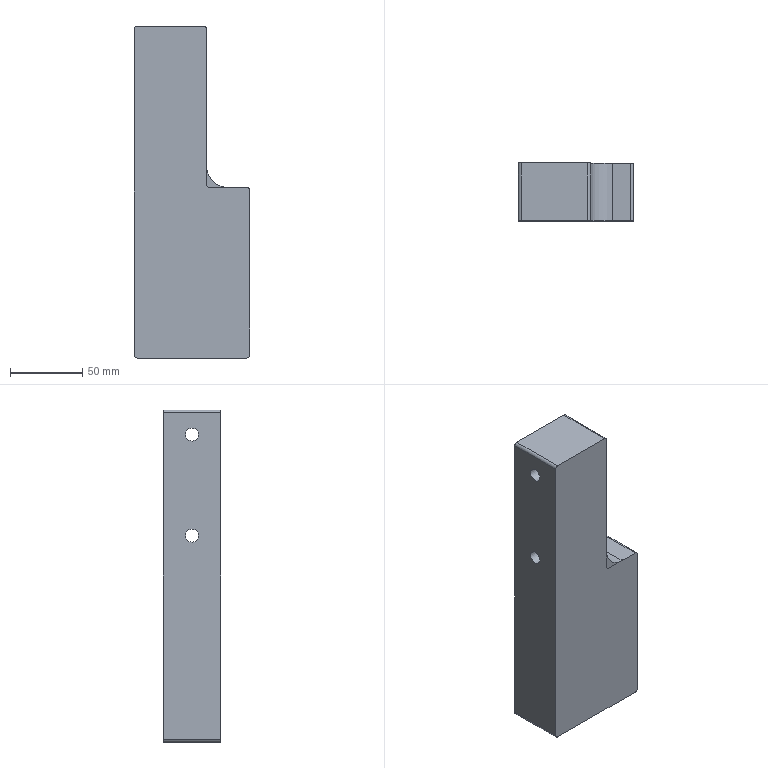CAM job | NX | 3+2 milling, drilling | part box 80 x 40 x 230 mm | stock box 80 x 50.5 x 230 mm
Tools:
number,name,description,diameter,corner_radius,flute_length,length,flutes
1,D16CU,Milling Tool-5 Parameters,16.0,0.0,50.0,75.0,2
3,D8点钻,Chamfer Mill,10.0,0.0,50.0,75.0,2
19,4倒角,Drilling Tool,4.0,0.0,35.0,50.0,2
2,D16.,Milling Tool-5 Parameters,16.0,0.0,50.0,75.0,2
20,D63精,Milling Tool-5 Parameters,63.0,0.0,50.0,75.0,2
18,D40.,Milling Tool-5 Parameters,40.0,0.0,50.0,75.0,2
1,D10.,Milling Tool-5 Parameters,10.0,0.0,50.0,75.0,2
10,Z6.8,Drilling Tool,6.8,0.0,35.0,50.0,2
11,M8,Drilling Tool,8.0,0.0,35.0,50.0,4
24,Z9.,Drilling Tool,9.0,0.0,35.0,50.0,2
5,D6.,Milling Tool-5 Parameters,6.0,0.0,50.0,75.0,2
23,D10R2.,Milling Tool-5 Parameters,10.0,2.0,50.0,75.0,2
Operations:
program,operation,operation_type,tool,method,geometry_group,spindle_rpm,surface_speed,feed_per_tooth,feed_cut,feed_plunge,cut_length_mm,path_length_mm,cut_time_min,machine_time_min
G54,FLOOR_FACING_COPY_2_1,VolumeBased25DMillingOperation,D40.,METHOD,WORKPIECE,1600.0,316.0,0.3125,1000.0,100.0,885.77,979.57,0.8858,0.8951
G54,PLANAR_MILL_COPY,PlanarMilling,D16CU,METHOD,WORKPIECE,1300.0,65.0,0.7692,2000.0,100.0,1856.0,6482.403,0.928,1.391
G54,PLANAR_MILL_COPY_COPY_2,PlanarMilling,D16CU,METHOD,WORKPIECE,1300.0,65.0,0.7692,2000.0,100.0,1856.0,6482.403,0.928,1.391
G54,ADAPTIVE_MILLING,CavityMilling,D16CU,METHOD,WORKPIECE,1300.0,65.0,0.7692,2000.0,100.0,49499.236,66202.841,16.172,17.842
G54,PLANAR_MILL_COPY_COPY_1_COPY,PlanarMilling,D16.,METHOD,WORKPIECE,1300.0,65.0,0.1923,500.0,100.0,665.967,846.267,1.332,1.35
G54,PLANAR_MILL_COPY_COPY_1_COPY_COPY,PlanarMilling,D16.,METHOD,WORKPIECE,800.0,40.0,0.25,400.0,100.0,1335.3,1515.6,3.338,3.356
G54,FLOOR_FACING_COPY_2_1_COPY,VolumeBased25DMillingOperation,D63精,METHOD,WORKPIECE,1600.0,316.0,0.125,400.0,100.0,650.418,744.418,1.626,1.635
G54,PLANAR_MILL_COPY_COPY_1,PlanarMilling,4倒角,METHOD,WORKPIECE,4500.0,113.0,0.0889,800.0,100.0,624.612,727.612,0.7808,0.7911
G54,PLANAR_MILL_COPY_COPY_1_COPY_1_COPY,PlanarMilling,D10.,METHOD,WORKPIECE_1,3500.0,109.0,0.2143,1500.0,100.0,2184.966,4081.568,1.457,1.646
G54,ADAPTIVE_MILLING_COPY,CavityMilling,D10.,METHOD,WORKPIECE_1,3500.0,109.0,0.5,3500.0,100.0,54185.283,54279.183,15.465,15.474
G54,FLOOR_FACING_COPY_2_1_COPY_1_COPY,VolumeBased25DMillingOperation,D63精,METHOD,WORKPIECE_1,1600.0,316.0,0.125,400.0,100.0,650.53,744.53,1.626,1.636
G54,PLANAR_MILL_COPY_COPY_1_COPY_1,PlanarMilling,4倒角,METHOD,WORKPIECE_1,4500.0,113.0,0.0889,800.0,100.0,626.612,729.612,0.7833,0.7936
PROGRAM_1,DRILLING_COPY,Operation,D8点钻,NONE,WORKPIECE_2,3500.0,87.0,0.0429,300.0,0.0,28.8,366.955,0.096,0.1298
PROGRAM_1,PECK_DRILLING,Operation,Z6.8,METHOD,WORKPIECE_2,1200.0,19.0,0.0333,80.0,0.0,72.0,337.05,0.9,0.9265
PROGRAM_1,PECK_DRILLING_COPY,Operation,M8,METHOD,WORKPIECE_2,200.0,5.0,0.0016,1.25,0.0,28.0,249.05,22.4,22.422
PROGRAM_1,PECK_DRILLING_COPY_1,Operation,Z9.,METHOD,WORKPIECE_2,1000.0,28.0,0.04,80.0,0.0,118.0,468.864,1.475,1.51
PROGRAM_1,HOLE_MILLING,CylinderMilling,D6.,METHOD,WORKPIECE_2,2700.0,50.0,0.1481,800.0,100.0,3578.274,3996.974,4.473,4.515
PROGRAM_1,HOLE_MILLING_COPY,CylinderMilling,D6.,METHOD,WORKPIECE_2,3000.0,56.0,0.01,60.0,100.0,84.823,534.823,1.414,1.459
PROGRAM_1,ZLEVEL_PROFILE_STEEP,ZLevelMilling,D16CU,METHOD,WORKPIECE_2,2600.0,130.0,0.4231,2200.0,100.0,4484.134,4644.106,2.038,2.054
PROGRAM_1,PLANAR_MILL,PlanarMilling,D10R2.,METHOD,WORKPIECE_2,2400.0,72.0,0.087,400.0,100.0,132.0,439.6,0.33,0.3608
PROGRAM_1,PLANAR_MILL_COPY_2,PlanarMilling,D10R2.,METHOD,WORKPIECE_2,2400.0,72.0,0.087,400.0,100.0,132.0,499.6,0.33,0.3668
PROGRAM_1,PLANAR_MILL_COPY_1,PlanarMilling,D10R2.,METHOD,WORKPIECE_2,2400.0,72.0,0.087,400.0,100.0,1240.8,2580.878,3.102,3.236
PROGRAM_2,DRILLING,Operation,D8点钻,METHOD,MCS_2,1000.0,25.0,0.04,80.0,0.0,9.0,111.09,0.1125,0.1227
PROGRAM_2,DRILLING_1,Operation,Z6.8,METHOD,MCS_2,1200.0,25.0,0.0333,80.0,0.0,66.0,225.09,0.825,0.8409
PROGRAM_2,PLANAR_MILL_1,PlanarMilling,D6.,METHOD,MCS_2,3500.0,65.0,0.1429,1000.0,100.0,1558.111,1603.111,1.558,1.563
PROGRAM_2,PLANAR_MILL_1_COPY,PlanarMilling,D6.,METHOD,MCS_2,2500.0,47.0,0.12,600.0,100.0,81.982,131.982,0.1366,0.1416
PROGRAM_2,PLANAR_MILL_2,PlanarMilling,D8点钻,METHOD,MCS_2,3000.0,75.0,0.1667,1000.0,100.0,42.853,82.853,0.0429,0.0469
PROGRAM_2,PLANAR_MILL_2_COPY,PlanarMilling,D8点钻,METHOD,MCS_2,3000.0,75.0,0.1667,1000.0,100.0,16.321,56.321,0.0163,0.0203
PROGRAM_2,PLANAR_MILL_2_COPY_COPY,PlanarMilling,D8点钻,METHOD,MCS_2,3000.0,75.0,0.1667,1000.0,100.0,16.321,70.321,0.0163,0.0217
PROGRAM_2,DRILLING_2,Operation,M8,METHOD,MCS_2,200.0,5.0,0.3125,250.0,0.0,9.0,58.0,0.036,0.0409
PROGRAM_2,DRILLING_2_COPY,Operation,M8,METHOD,MCS_2,200.0,5.0,0.3125,250.0,0.0,16.0,72.0,0.064,0.0696